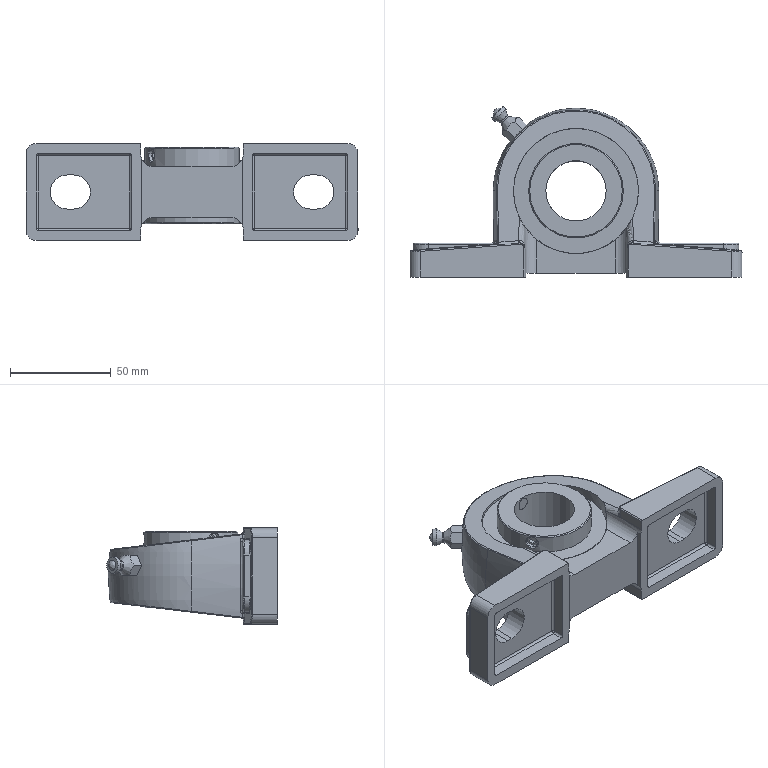Part | STEP file | GBT7810-1995-UCP206 | 1 solid | 240 faces | box 165 x 84.83 x 48 mm | volume 210278 mm3 | cylinder 81 | spline 78 | plane 72 | cone 8 | torus 1 | commonest cylinder face diameters 1 x22 2 x16 3 x8 6 x6 4 x4 10 x4